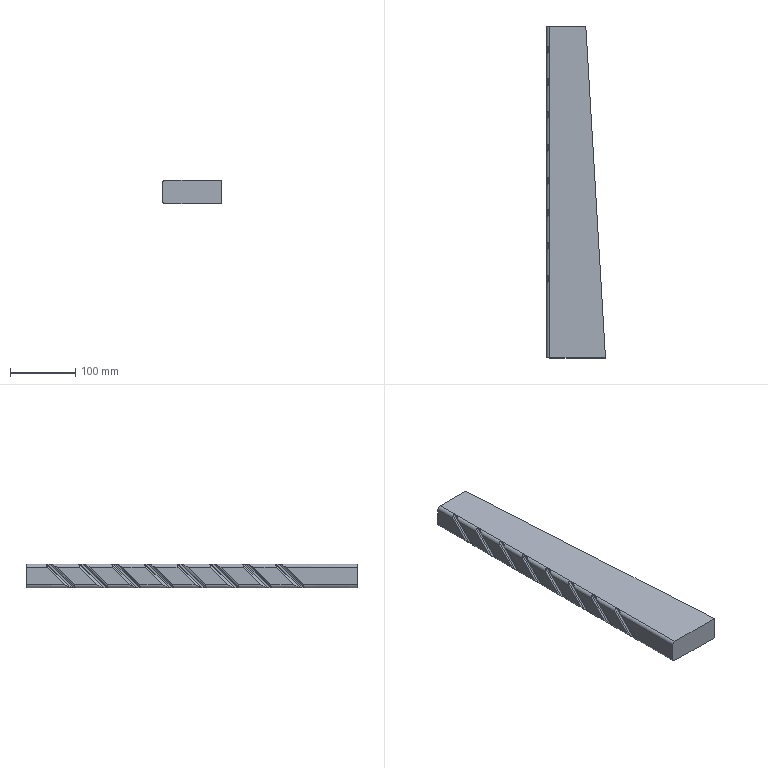Part | STEP file | 03-High-level comb rack 1 | 1 solid | 56 faces | box 90 x 507 x 36 mm | volume 1352906 mm3 | cylinder 34 | plane 22 | commonest cylinder face diameters 4 x32 10 x2